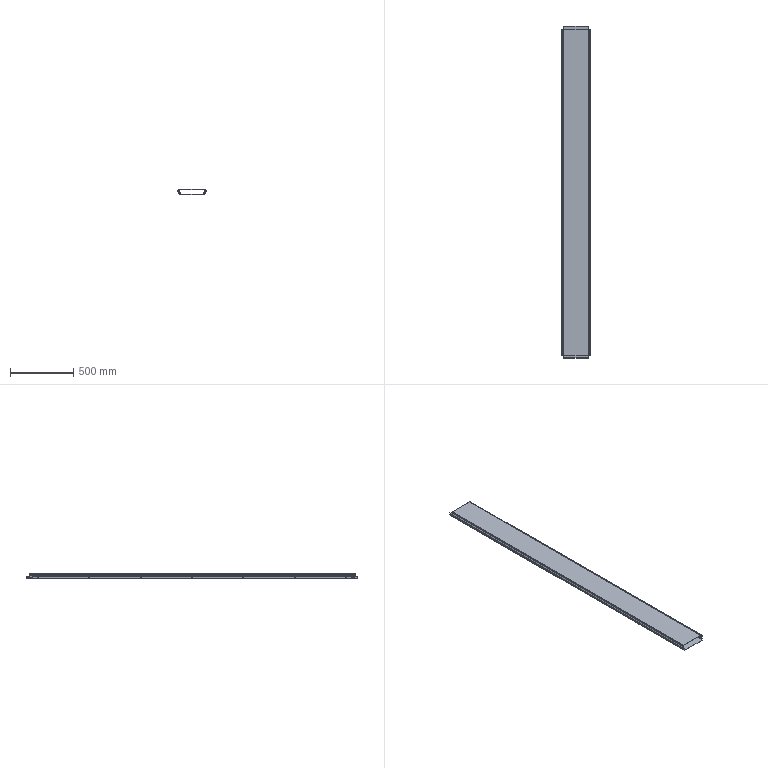Part | 18 solids | 495 faces | box 227 x 2616 x 41 mm | volume 2325398 mm3 | plane 292 | cylinder 203 | commonest cylinder face diameters 6 x28 6.2 x28 8 x28 12 x28 6.4 x24 0.6 x20